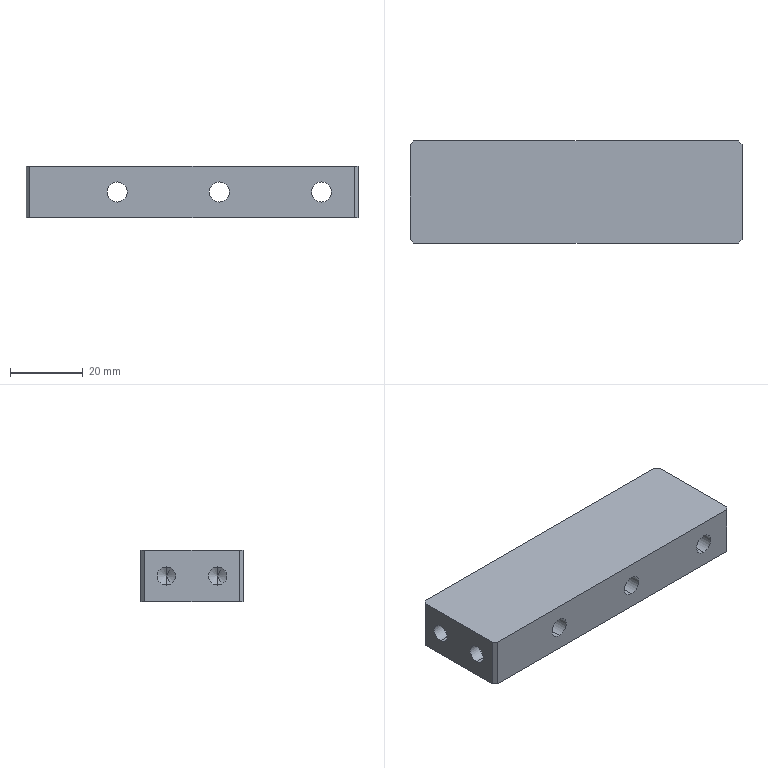Part | SolidWorks | features HoleWzd 2, Chamfer 1, Extrusion 1 | 1 solid | 33 faces | box 91 x 28 x 14 mm | volume 31396 mm3 | cylinder 16 | plane 13 | cone 4 | commonest cylinder face diameters 5.5 x6 10 x6 5 x4
STEP:
#1=CARTESIAN_POINT('',(-20.5,4.,-5.));
#2=VERTEX_POINT('',#1);
#3=CARTESIAN_POINT('',(-20.5,4.,5.));
#4=VERTEX_POINT('',#3);
#5=CARTESIAN_POINT('',(-20.5,4.,0.));
#6=DIRECTION('',(0.,1.,0.));
#7=DIRECTION('',(0.,0.,1.));
#8=AXIS2_PLACEMENT_3D('',#5,#6,#7);
#9=CIRCLE('',#8,5.);
#10=EDGE_CURVE('',#2,#4,#9,.T.);
#11=ORIENTED_EDGE('',*,*,#10,.F.);
#12=CARTESIAN_POINT('',(-20.5,14.,-5.));
#13=VERTEX_POINT('',#12);
#14=CARTESIAN_POINT('',(-20.5,14.,-5.));
#15=DIRECTION('',(0.,1.,0.));
#16=VECTOR('',#15,1000.);
#17=LINE('',#14,#16);
#18=EDGE_CURVE('',#2,#13,#17,.T.);
#19=ORIENTED_EDGE('',*,*,#18,.T.);
#20=CARTESIAN_POINT('',(-20.5,14.,5.));
#21=VERTEX_POINT('',#20);
#22=CARTESIAN_POINT('',(-20.5,14.,0.));
#23=DIRECTION('',(0.,1.,0.));
#24=DIRECTION('',(0.,0.,1.));
#25=AXIS2_PLACEMENT_3D('',#22,#23,#24);
#26=CIRCLE('',#25,5.);
#27=EDGE_CURVE('',#13,#21,#26,.T.);
#28=ORIENTED_EDGE('',*,*,#27,.T.);
#29=CARTESIAN_POINT('',(-20.5,14.,5.));
#30=DIRECTION('',(0.,1.,0.));
#31=VECTOR('',#30,1000.);
#32=LINE('',#29,#31);
#33=EDGE_CURVE('',#4,#21,#32,.T.);
#34=ORIENTED_EDGE('',*,*,#33,.F.);
#35=EDGE_LOOP('',(#11,#19,#28,#34));
#36=FACE_OUTER_BOUND('',#35,.T.);
#37=CARTESIAN_POINT('',(-20.5,14.,0.));
#38=DIRECTION('',(0.,1.,0.));
#39=DIRECTION('',(0.,0.,1.));
#40=AXIS2_PLACEMENT_3D('',#37,#38,#39);
#41=CYLINDRICAL_SURFACE('',#40,5.);
#42=ADVANCED_FACE('',(#36),#41,.F.);
#43=CARTESIAN_POINT('',(-20.5,-14.,-2.75));
#44=VERTEX_POINT('',#43);
#45=CARTESIAN_POINT('',(-20.5,-14.,2.75));
#46=VERTEX_POINT('',#45);
#47=CARTESIAN_POINT('',(-20.5,-14.,0.));
#48=DIRECTION('',(0.,1.,0.));
#49=DIRECTION('',(0.,0.,1.));
#50=AXIS2_PLACEMENT_3D('',#47,#48,#49);
#51=CIRCLE('',#50,2.75);
#52=EDGE_CURVE('',#44,#46,#51,.T.);
#53=ORIENTED_EDGE('',*,*,#52,.F.);
#54=CARTESIAN_POINT('',(-20.5,4.,-2.75));
#55=VERTEX_POINT('',#54);
#56=CARTESIAN_POINT('',(-20.5,14.,-2.75));
#57=DIRECTION('',(0.,1.,0.));
#58=VECTOR('',#57,1000.);
#59=LINE('',#56,#58);
#60=EDGE_CURVE('',#44,#55,#59,.T.);
#61=ORIENTED_EDGE('',*,*,#60,.T.);
#62=CARTESIAN_POINT('',(-20.5,4.,2.75));
#63=VERTEX_POINT('',#62);
#64=CARTESIAN_POINT('',(-20.5,4.,0.));
#65=DIRECTION('',(0.,1.,0.));
#66=DIRECTION('',(0.,0.,1.));
#67=AXIS2_PLACEMENT_3D('',#64,#65,#66);
#68=CIRCLE('',#67,2.75);
#69=EDGE_CURVE('',#55,#63,#68,.T.);
#70=ORIENTED_EDGE('',*,*,#69,.T.);
#71=CARTESIAN_POINT('',(-20.5,14.,2.75));
#72=DIRECTION('',(0.,1.,0.));
#73=VECTOR('',#72,1000.);
#74=LINE('',#71,#73);
#75=EDGE_CURVE('',#46,#63,#74,.T.);
#76=ORIENTED_EDGE('',*,*,#75,.F.);
#77=EDGE_LOOP('',(#53,#61,#70,#76));
#78=FACE_OUTER_BOUND('',#77,.T.);
#79=CARTESIAN_POINT('',(-20.5,14.,0.));
#80=DIRECTION('',(0.,1.,0.));
#81=DIRECTION('',(0.,0.,1.));
#82=AXIS2_PLACEMENT_3D('',#79,#80,#81);
#83=CYLINDRICAL_SURFACE('',#82,2.75);
#84=ADVANCED_FACE('',(#78),#83,.F.);
#85=CARTESIAN_POINT('',(35.5,4.,-5.));
#86=VERTEX_POINT('',#85);
#87=CARTESIAN_POINT('',(35.5,4.,5.));
#88=VERTEX_POINT('',#87);
#89=CARTESIAN_POINT('',(35.5,4.,0.));
#90=DIRECTION('',(0.,1.,0.));
#91=DIRECTION('',(0.,0.,1.));
#92=AXIS2_PLACEMENT_3D('',#89,#90,#91);
#93=CIRCLE('',#92,5.);
#94=EDGE_CURVE('',#86,#88,#93,.T.);
#95=ORIENTED_EDGE('',*,*,#94,.F.);
#96=CARTESIAN_POINT('',(35.5,14.,-5.));
#97=VERTEX_POINT('',#96);
#98=CARTESIAN_POINT('',(35.5,14.,-5.));
#99=DIRECTION('',(0.,1.,0.));
#100=VECTOR('',#99,1000.);
#101=LINE('',#98,#100);
#102=EDGE_CURVE('',#86,#97,#101,.T.);
#103=ORIENTED_EDGE('',*,*,#102,.T.);
#104=CARTESIAN_POINT('',(35.5,14.,5.));
#105=VERTEX_POINT('',#104);
#106=CARTESIAN_POINT('',(35.5,14.,0.));
#107=DIRECTION('',(0.,1.,0.));
#108=DIRECTION('',(0.,0.,1.));
#109=AXIS2_PLACEMENT_3D('',#106,#107,#108);
#110=CIRCLE('',#109,5.);
#111=EDGE_CURVE('',#97,#105,#110,.T.);
#112=ORIENTED_EDGE('',*,*,#111,.T.);
#113=CARTESIAN_POINT('',(35.5,14.,5.));
#114=DIRECTION('',(0.,1.,0.));
#115=VECTOR('',#114,1000.);
#116=LINE('',#113,#115);
#117=EDGE_CURVE('',#88,#105,#116,.T.);
#118=ORIENTED_EDGE('',*,*,#117,.F.);
#119=EDGE_LOOP('',(#95,#103,#112,#118));
#120=FACE_OUTER_BOUND('',#119,.T.);
#121=CARTESIAN_POINT('',(35.5,14.,0.));
#122=DIRECTION('',(0.,1.,0.));
#123=DIRECTION('',(0.,0.,1.));
#124=AXIS2_PLACEMENT_3D('',#121,#122,#123);
#125=CYLINDRICAL_SURFACE('',#124,5.);
#126=ADVANCED_FACE('',(#120),#125,.F.);
#127=CARTESIAN_POINT('',(35.5,-14.,-2.75));
#128=VERTEX_POINT('',#127);
#129=CARTESIAN_POINT('',(35.5,-14.,2.75));
#130=VERTEX_POINT('',#129);
#131=CARTESIAN_POINT('',(35.5,-14.,0.));
#132=DIRECTION('',(0.,1.,0.));
#133=DIRECTION('',(0.,0.,1.));
#134=AXIS2_PLACEMENT_3D('',#131,#132,#133);
#135=CIRCLE('',#134,2.75);
#136=EDGE_CURVE('',#128,#130,#135,.T.);
#137=ORIENTED_EDGE('',*,*,#136,.F.);
#138=CARTESIAN_POINT('',(35.5,4.,-2.75));
#139=VERTEX_POINT('',#138);
#140=CARTESIAN_POINT('',(35.5,14.,-2.75));
#141=DIRECTION('',(0.,1.,0.));
#142=VECTOR('',#141,1000.);
#143=LINE('',#140,#142);
#144=EDGE_CURVE('',#128,#139,#143,.T.);
#145=ORIENTED_EDGE('',*,*,#144,.T.);
#146=CARTESIAN_POINT('',(35.5,4.,2.75));
#147=VERTEX_POINT('',#146);
#148=CARTESIAN_POINT('',(35.5,4.,0.));
#149=DIRECTION('',(0.,1.,0.));
#150=DIRECTION('',(0.,0.,1.));
#151=AXIS2_PLACEMENT_3D('',#148,#149,#150);
#152=CIRCLE('',#151,2.75);
#153=EDGE_CURVE('',#139,#147,#152,.T.);
#154=ORIENTED_EDGE('',*,*,#153,.T.);
#155=CARTESIAN_POINT('',(35.5,14.,2.75));
#156=DIRECTION('',(0.,1.,0.));
#157=VECTOR('',#156,1000.);
#158=LINE('',#155,#157);
#159=EDGE_CURVE('',#130,#147,#158,.T.);
#160=ORIENTED_EDGE('',*,*,#159,.F.);
#161=EDGE_LOOP('',(#137,#145,#154,#160));
#162=FACE_OUTER_BOUND('',#161,.T.);
#163=CARTESIAN_POINT('',(35.5,14.,0.));
#164=DIRECTION('',(0.,1.,0.));
#165=DIRECTION('',(0.,0.,1.));
#166=AXIS2_PLACEMENT_3D('',#163,#164,#165);
#167=CYLINDRICAL_SURFACE('',#166,2.75);
#168=ADVANCED_FACE('',(#162),#167,.F.);
#169=CARTESIAN_POINT('',(7.5,4.,-5.));
#170=VERTEX_POINT('',#169);
#171=CARTESIAN_POINT('',(7.5,4.,5.));
#172=VERTEX_POINT('',#171);
#173=CARTESIAN_POINT('',(7.5,4.,0.));
#174=DIRECTION('',(0.,1.,0.));
#175=DIRECTION('',(0.,0.,1.));
#176=AXIS2_PLACEMENT_3D('',#173,#174,#175);
#177=CIRCLE('',#176,5.);
#178=EDGE_CURVE('',#170,#172,#177,.T.);
#179=ORIENTED_EDGE('',*,*,#178,.F.);
#180=CARTESIAN_POINT('',(7.5,14.,-5.));
#181=VERTEX_POINT('',#180);
#182=CARTESIAN_POINT('',(7.5,14.,-5.));
#183=DIRECTION('',(0.,1.,0.));
#184=VECTOR('',#183,1000.);
#185=LINE('',#182,#184);
#186=EDGE_CURVE('',#170,#181,#185,.T.);
#187=ORIENTED_EDGE('',*,*,#186,.T.);
#188=CARTESIAN_POINT('',(7.5,14.,5.));
#189=VERTEX_POINT('',#188);
#190=CARTESIAN_POINT('',(7.5,14.,0.));
#191=DIRECTION('',(0.,1.,0.));
#192=DIRECTION('',(0.,0.,1.));
#193=AXIS2_PLACEMENT_3D('',#190,#191,#192);
#194=CIRCLE('',#193,5.);
#195=EDGE_CURVE('',#181,#189,#194,.T.);
#196=ORIENTED_EDGE('',*,*,#195,.T.);
#197=CARTESIAN_POINT('',(7.5,14.,5.));
#198=DIRECTION('',(0.,1.,0.));
#199=VECTOR('',#198,1000.);
#200=LINE('',#197,#199);
#201=EDGE_CURVE('',#172,#189,#200,.T.);
#202=ORIENTED_EDGE('',*,*,#201,.F.);
#203=EDGE_LOOP('',(#179,#187,#196,#202));
#204=FACE_OUTER_BOUND('',#203,.T.);
#205=CARTESIAN_POINT('',(7.5,14.,0.));
#206=DIRECTION('',(0.,1.,0.));
#207=DIRECTION('',(0.,0.,1.));
#208=AXIS2_PLACEMENT_3D('',#205,#206,#207);
#209=CYLINDRICAL_SURFACE('',#208,5.);
#210=ADVANCED_FACE('',(#204),#209,.F.);
#211=CARTESIAN_POINT('',(7.5,-14.,-2.75));
#212=VERTEX_POINT('',#211);
#213=CARTESIAN_POINT('',(7.5,-14.,2.75));
#214=VERTEX_POINT('',#213);
#215=CARTESIAN_POINT('',(7.5,-14.,0.));
#216=DIRECTION('',(0.,1.,0.));
#217=DIRECTION('',(0.,0.,1.));
#218=AXIS2_PLACEMENT_3D('',#215,#216,#217);
#219=CIRCLE('',#218,2.75);
#220=EDGE_CURVE('',#212,#214,#219,.T.);
#221=ORIENTED_EDGE('',*,*,#220,.F.);
#222=CARTESIAN_POINT('',(7.5,4.,-2.75));
#223=VERTEX_POINT('',#222);
#224=CARTESIAN_POINT('',(7.5,14.,-2.75));
#225=DIRECTION('',(0.,1.,0.));
#226=VECTOR('',#225,1000.);
#227=LINE('',#224,#226);
#228=EDGE_CURVE('',#212,#223,#227,.T.);
#229=ORIENTED_EDGE('',*,*,#228,.T.);
#230=CARTESIAN_POINT('',(7.5,4.,2.75));
#231=VERTEX_POINT('',#230);
#232=CARTESIAN_POINT('',(7.5,4.,0.));
#233=DIRECTION('',(0.,1.,0.));
#234=DIRECTION('',(0.,0.,1.));
#235=AXIS2_PLACEMENT_3D('',#232,#233,#234);
#236=CIRCLE('',#235,2.75);
#237=EDGE_CURVE('',#223,#231,#236,.T.);
#238=ORIENTED_EDGE('',*,*,#237,.T.);
#239=CARTESIAN_POINT('',(7.5,14.,2.75));
#240=DIRECTION('',(0.,1.,0.));
#241=VECTOR('',#240,1000.);
#242=LINE('',#239,#241);
#243=EDGE_CURVE('',#214,#231,#242,.T.);
#244=ORIENTED_EDGE('',*,*,#243,.F.);
#245=EDGE_LOOP('',(#221,#229,#238,#244));
#246=FACE_OUTER_BOUND('',#245,.T.);
#247=CARTESIAN_POINT('',(7.5,14.,0.));
#248=DIRECTION('',(0.,1.,0.));
#249=DIRECTION('',(0.,0.,1.));
#250=AXIS2_PLACEMENT_3D('',#247,#248,#249);
#251=CYLINDRICAL_SURFACE('',#250,2.75);
#252=ADVANCED_FACE('',(#246),#251,.F.);
#253=CARTESIAN_POINT('',(-30.5,7.,-2.5));
#254=VERTEX_POINT('',#253);
#255=CARTESIAN_POINT('',(-30.5,7.,2.5));
#256=VERTEX_POINT('',#255);
#257=CARTESIAN_POINT('',(-30.5,7.,0.));
#258=DIRECTION('',(-1.,0.,0.));
#259=DIRECTION('',(0.,0.,1.));
#260=AXIS2_PLACEMENT_3D('',#257,#258,#259);
#261=CIRCLE('',#260,2.5);
#262=EDGE_CURVE('',#254,#256,#261,.T.);
#263=ORIENTED_EDGE('',*,*,#262,.F.);
#264=CARTESIAN_POINT('',(-45.5,7.,-2.5));
#265=VERTEX_POINT('',#264);
#266=CARTESIAN_POINT('',(-45.5,7.,-2.5));
#267=DIRECTION('',(-1.,0.,0.));
#268=VECTOR('',#267,1000.);
#269=LINE('',#266,#268);
#270=EDGE_CURVE('',#254,#265,#269,.T.);
#271=ORIENTED_EDGE('',*,*,#270,.T.);
#272=CARTESIAN_POINT('',(-45.5,7.,2.5));
#273=VERTEX_POINT('',#272);
#274=CARTESIAN_POINT('',(-45.5,7.,0.));
#275=DIRECTION('',(-1.,0.,0.));
#276=DIRECTION('',(0.,0.,1.));
#277=AXIS2_PLACEMENT_3D('',#274,#275,#276);
#278=CIRCLE('',#277,2.5);
#279=EDGE_CURVE('',#265,#273,#278,.T.);
#280=ORIENTED_EDGE('',*,*,#279,.T.);
#281=CARTESIAN_POINT('',(-45.5,7.,2.5));
#282=DIRECTION('',(-1.,0.,0.));
#283=VECTOR('',#282,1000.);
#284=LINE('',#281,#283);
#285=EDGE_CURVE('',#256,#273,#284,.T.);
#286=ORIENTED_EDGE('',*,*,#285,.F.);
#287=EDGE_LOOP('',(#263,#271,#280,#286));
#288=FACE_OUTER_BOUND('',#287,.T.);
#289=CARTESIAN_POINT('',(-45.5,7.,0.));
#290=DIRECTION('',(-1.,0.,0.));
#291=DIRECTION('',(0.,0.,1.));
#292=AXIS2_PLACEMENT_3D('',#289,#290,#291);
#293=CYLINDRICAL_SURFACE('',#292,2.5);
#294=ADVANCED_FACE('',(#288),#293,.F.);
#295=CARTESIAN_POINT('',(-28.998,7.,0.));
#296=VERTEX_POINT('',#295);
#297=CARTESIAN_POINT('',(-30.5,7.,2.5));
#298=DIRECTION('',(-0.515,0.,0.8572));
#299=VECTOR('',#298,1000.);
#300=LINE('',#297,#299);
#301=EDGE_CURVE('',#296,#256,#300,.T.);
#302=ORIENTED_EDGE('',*,*,#301,.F.);
#303=CARTESIAN_POINT('',(-30.5,7.,-2.5));
#304=DIRECTION('',(-0.515,0.,-0.8572));
#305=VECTOR('',#304,1000.);
#306=LINE('',#303,#305);
#307=EDGE_CURVE('',#296,#254,#306,.T.);
#308=ORIENTED_EDGE('',*,*,#307,.T.);
#309=ORIENTED_EDGE('',*,*,#262,.T.);
#310=EDGE_LOOP('',(#302,#308,#309));
#311=FACE_OUTER_BOUND('',#310,.T.);
#312=CARTESIAN_POINT('',(-30.5,7.,0.));
#313=DIRECTION('',(-1.,0.,0.));
#314=DIRECTION('',(0.,0.,1.));
#315=AXIS2_PLACEMENT_3D('',#312,#313,#314);
#316=CONICAL_SURFACE('',#315,2.5,1.03);
#317=ADVANCED_FACE('',(#311),#316,.F.);
#318=CARTESIAN_POINT('',(-30.5,-7.,-2.5));
#319=VERTEX_POINT('',#318);
#320=CARTESIAN_POINT('',(-30.5,-7.,2.5));
#321=VERTEX_POINT('',#320);
#322=CARTESIAN_POINT('',(-30.5,-7.,0.));
#323=DIRECTION('',(-1.,0.,0.));
#324=DIRECTION('',(0.,0.,1.));
#325=AXIS2_PLACEMENT_3D('',#322,#323,#324);
#326=CIRCLE('',#325,2.5);
#327=EDGE_CURVE('',#319,#321,#326,.T.);
#328=ORIENTED_EDGE('',*,*,#327,.F.);
#329=CARTESIAN_POINT('',(-45.5,-7.,-2.5));
#330=VERTEX_POINT('',#329);
#331=CARTESIAN_POINT('',(-45.5,-7.,-2.5));
#332=DIRECTION('',(-1.,0.,0.));
#333=VECTOR('',#332,1000.);
#334=LINE('',#331,#333);
#335=EDGE_CURVE('',#319,#330,#334,.T.);
#336=ORIENTED_EDGE('',*,*,#335,.T.);
#337=CARTESIAN_POINT('',(-45.5,-7.,2.5));
#338=VERTEX_POINT('',#337);
#339=CARTESIAN_POINT('',(-45.5,-7.,0.));
#340=DIRECTION('',(-1.,0.,0.));
#341=DIRECTION('',(0.,0.,1.));
#342=AXIS2_PLACEMENT_3D('',#339,#340,#341);
#343=CIRCLE('',#342,2.5);
#344=EDGE_CURVE('',#330,#338,#343,.T.);
#345=ORIENTED_EDGE('',*,*,#344,.T.);
#346=CARTESIAN_POINT('',(-45.5,-7.,2.5));
#347=DIRECTION('',(-1.,0.,0.));
#348=VECTOR('',#347,1000.);
#349=LINE('',#346,#348);
#350=EDGE_CURVE('',#321,#338,#349,.T.);
#351=ORIENTED_EDGE('',*,*,#350,.F.);
#352=EDGE_LOOP('',(#328,#336,#345,#351));
#353=FACE_OUTER_BOUND('',#352,.T.);
#354=CARTESIAN_POINT('',(-45.5,-7.,0.));
#355=DIRECTION('',(-1.,0.,0.));
#356=DIRECTION('',(0.,0.,1.));
#357=AXIS2_PLACEMENT_3D('',#354,#355,#356);
#358=CYLINDRICAL_SURFACE('',#357,2.5);
#359=ADVANCED_FACE('',(#353),#358,.F.);
#360=CARTESIAN_POINT('',(-28.998,-7.,0.));
#361=VERTEX_POINT('',#360);
#362=CARTESIAN_POINT('',(-30.5,-7.,2.5));
#363=DIRECTION('',(-0.515,0.,0.8572));
#364=VECTOR('',#363,1000.);
#365=LINE('',#362,#364);
#366=EDGE_CURVE('',#361,#321,#365,.T.);
#367=ORIENTED_EDGE('',*,*,#366,.F.);
#368=CARTESIAN_POINT('',(-30.5,-7.,-2.5));
#369=DIRECTION('',(-0.515,0.,-0.8572));
#370=VECTOR('',#369,1000.);
#371=LINE('',#368,#370);
#372=EDGE_CURVE('',#361,#319,#371,.T.);
#373=ORIENTED_EDGE('',*,*,#372,.T.);
#374=ORIENTED_EDGE('',*,*,#327,.T.);
#375=EDGE_LOOP('',(#367,#373,#374));
#376=FACE_OUTER_BOUND('',#375,.T.);
#377=CARTESIAN_POINT('',(-30.5,-7.,0.));
#378=DIRECTION('',(-1.,0.,0.));
#379=DIRECTION('',(0.,0.,1.));
#380=AXIS2_PLACEMENT_3D('',#377,#378,#379);
#381=CONICAL_SURFACE('',#380,2.5,1.03);
#382=ADVANCED_FACE('',(#376),#381,.F.);
#383=CARTESIAN_POINT('',(45.5,-13.,-7.));
#384=VERTEX_POINT('',#383);
#385=CARTESIAN_POINT('',(45.5,13.,-7.));
#386=VERTEX_POINT('',#385);
#387=CARTESIAN_POINT('',(45.5,-14.,-7.));
#388=DIRECTION('',(0.,1.,0.));
#389=VECTOR('',#388,1000.);
#390=LINE('',#387,#389);
#391=EDGE_CURVE('',#384,#386,#390,.T.);
#392=ORIENTED_EDGE('',*,*,#391,.T.);
#393=CARTESIAN_POINT('',(45.5,13.,7.));
#394=VERTEX_POINT('',#393);
#395=CARTESIAN_POINT('',(45.5,13.,7.));
#396=DIRECTION('',(0.,0.,1.));
#397=VECTOR('',#396,1000.);
#398=LINE('',#395,#397);
#399=EDGE_CURVE('',#386,#394,#398,.T.);
#400=ORIENTED_EDGE('',*,*,#399,.T.);
#401=CARTESIAN_POINT('',(45.5,-13.,7.));
#402=VERTEX_POINT('',#401);
#403=CARTESIAN_POINT('',(45.5,-14.,7.));
#404=DIRECTION('',(0.,1.,0.));
#405=VECTOR('',#404,1000.);
#406=LINE('',#403,#405);
#407=EDGE_CURVE('',#402,#394,#406,.T.);
#408=ORIENTED_EDGE('',*,*,#407,.F.);
#409=CARTESIAN_POINT('',(45.5,-13.,7.));
#410=DIRECTION('',(0.,0.,-1.));
#411=VECTOR('',#410,1000.);
#412=LINE('',#409,#411);
#413=EDGE_CURVE('',#402,#384,#412,.T.);
#414=ORIENTED_EDGE('',*,*,#413,.T.);
#415=EDGE_LOOP('',(#392,#400,#408,#414));
#416=FACE_OUTER_BOUND('',#415,.T.);
#417=CARTESIAN_POINT('',(45.5,-14.,7.));
#418=DIRECTION('',(-1.,0.,0.));
#419=DIRECTION('',(0.,0.,1.));
#420=AXIS2_PLACEMENT_3D('',#417,#418,#419);
#421=PLANE('',#420);
#422=ADVANCED_FACE('',(#416),#421,.F.);
#423=CARTESIAN_POINT('',(-20.5,14.,0.));
#424=DIRECTION('',(0.,1.,0.));
#425=DIRECTION('',(0.,0.,1.));
#426=AXIS2_PLACEMENT_3D('',#423,#424,#425);
#427=CIRCLE('',#426,5.);
#428=EDGE_CURVE('',#21,#13,#427,.T.);
#429=ORIENTED_EDGE('',*,*,#428,.F.);
#430=ORIENTED_EDGE('',*,*,#27,.F.);
#431=EDGE_LOOP('',(#429,#430));
#432=FACE_BOUND('',#431,.T.);
#433=CARTESIAN_POINT('',(35.5,14.,0.));
#434=DIRECTION('',(0.,1.,0.));
#435=DIRECTION('',(0.,0.,1.));
#436=AXIS2_PLACEMENT_3D('',#433,#434,#435);
#437=CIRCLE('',#436,5.);
#438=EDGE_CURVE('',#105,#97,#437,.T.);
#439=ORIENTED_EDGE('',*,*,#438,.F.);
#440=ORIENTED_EDGE('',*,*,#111,.F.);
#441=EDGE_LOOP('',(#439,#440));
#442=FACE_BOUND('',#441,.T.);
#443=CARTESIAN_POINT('',(7.5,14.,0.));
#444=DIRECTION('',(0.,1.,0.));
#445=DIRECTION('',(0.,0.,1.));
#446=AXIS2_PLACEMENT_3D('',#443,#444,#445);
#447=CIRCLE('',#446,5.);
#448=EDGE_CURVE('',#189,#181,#447,.T.);
#449=ORIENTED_EDGE('',*,*,#448,.F.);
#450=ORIENTED_EDGE('',*,*,#195,.F.);
#451=EDGE_LOOP('',(#449,#450));
#452=FACE_BOUND('',#451,.T.);
#453=CARTESIAN_POINT('',(44.5,14.,7.));
#454=VERTEX_POINT('',#453);
#455=CARTESIAN_POINT('',(-44.5,14.,7.));
#456=VERTEX_POINT('',#455);
#457=CARTESIAN_POINT('',(-45.5,14.,7.));
#458=DIRECTION('',(-1.,0.,0.));
#459=VECTOR('',#458,1000.);
#460=LINE('',#457,#459);
#461=EDGE_CURVE('',#454,#456,#460,.T.);
#462=ORIENTED_EDGE('',*,*,#461,.F.);
#463=CARTESIAN_POINT('',(44.5,14.,-7.));
#464=VERTEX_POINT('',#463);
#465=CARTESIAN_POINT('',(44.5,14.,7.));
#466=DIRECTION('',(0.,0.,-1.));
#467=VECTOR('',#466,1000.);
#468=LINE('',#465,#467);
#469=EDGE_CURVE('',#454,#464,#468,.T.);
#470=ORIENTED_EDGE('',*,*,#469,.T.);
#471=CARTESIAN_POINT('',(-44.5,14.,-7.));
#472=VERTEX_POINT('',#471);
#473=CARTESIAN_POINT('',(-45.5,14.,-7.));
#474=DIRECTION('',(-1.,0.,0.));
#475=VECTOR('',#474,1000.);
#476=LINE('',#473,#475);
#477=EDGE_CURVE('',#464,#472,#476,.T.);
#478=ORIENTED_EDGE('',*,*,#477,.T.);
#479=CARTESIAN_POINT('',(-44.5,14.,7.));
#480=DIRECTION('',(0.,0.,1.));
#481=VECTOR('',#480,1000.);
#482=LINE('',#479,#481);
#483=EDGE_CURVE('',#472,#456,#482,.T.);
#484=ORIENTED_EDGE('',*,*,#483,.T.);
#485=EDGE_LOOP('',(#462,#470,#478,#484));
#486=FACE_OUTER_BOUND('',#485,.T.);
#487=CARTESIAN_POINT('',(-45.5,14.,7.));
#488=DIRECTION('',(0.,-1.,0.));
#489=DIRECTION('',(0.,0.,-1.));
#490=AXIS2_PLACEMENT_3D('',#487,#488,#489);
#491=PLANE('',#490);
#492=ADVANCED_FACE('',(#432,#442,#452,#486),#491,.F.);
#493=CARTESIAN_POINT('',(-45.5,7.,0.));
#494=DIRECTION('',(-1.,0.,0.));
#495=DIRECTION('',(0.,0.,1.));
#496=AXIS2_PLACEMENT_3D('',#493,#494,#495);
#497=CIRCLE('',#496,2.5);
#498=EDGE_CURVE('',#273,#265,#497,.T.);
#499=ORIENTED_EDGE('',*,*,#498,.F.);
#500=ORIENTED_EDGE('',*,*,#279,.F.);
#501=EDGE_LOOP('',(#499,#500));
#502=FACE_BOUND('',#501,.T.);
#503=CARTESIAN_POINT('',(-45.5,-7.,0.));
#504=DIRECTION('',(-1.,0.,0.));
#505=DIRECTION('',(0.,0.,1.));
#506=AXIS2_PLACEMENT_3D('',#503,#504,#505);
#507=CIRCLE('',#506,2.5);
#508=EDGE_CURVE('',#338,#330,#507,.T.);
#509=ORIENTED_EDGE('',*,*,#508,.F.);
#510=ORIENTED_EDGE('',*,*,#344,.F.);
#511=EDGE_LOOP('',(#509,#510));
#512=FACE_BOUND('',#511,.T.);
#513=CARTESIAN_POINT('',(-45.5,13.,-7.));
#514=VERTEX_POINT('',#513);
#515=CARTESIAN_POINT('',(-45.5,-13.,-7.));
#516=VERTEX_POINT('',#515);
#517=CARTESIAN_POINT('',(-45.5,-14.,-7.));
#518=DIRECTION('',(0.,-1.,0.));
#519=VECTOR('',#518,1000.);
#520=LINE('',#517,#519);
#521=EDGE_CURVE('',#514,#516,#520,.T.);
#522=ORIENTED_EDGE('',*,*,#521,.T.);
#523=CARTESIAN_POINT('',(-45.5,-13.,7.));
#524=VERTEX_POINT('',#523);
#525=CARTESIAN_POINT('',(-45.5,-13.,7.));
#526=DIRECTION('',(0.,0.,1.));
#527=VECTOR('',#526,1000.);
#528=LINE('',#525,#527);
#529=EDGE_CURVE('',#516,#524,#528,.T.);
#530=ORIENTED_EDGE('',*,*,#529,.T.);
#531=CARTESIAN_POINT('',(-45.5,13.,7.));
#532=VERTEX_POINT('',#531);
#533=CARTESIAN_POINT('',(-45.5,-14.,7.));
#534=DIRECTION('',(0.,-1.,0.));
#535=VECTOR('',#534,1000.);
#536=LINE('',#533,#535);
#537=EDGE_CURVE('',#532,#524,#536,.T.);
#538=ORIENTED_EDGE('',*,*,#537,.F.);
#539=CARTESIAN_POINT('',(-45.5,13.,7.));
#540=DIRECTION('',(0.,0.,-1.));
#541=VECTOR('',#540,1000.);
#542=LINE('',#539,#541);
#543=EDGE_CURVE('',#532,#514,#542,.T.);
#544=ORIENTED_EDGE('',*,*,#543,.T.);
#545=EDGE_LOOP('',(#522,#530,#538,#544));
#546=FACE_OUTER_BOUND('',#545,.T.);
#547=CARTESIAN_POINT('',(-45.5,-14.,7.));
#548=DIRECTION('',(1.,0.,0.));
#549=DIRECTION('',(0.,0.,-1.));
#550=AXIS2_PLACEMENT_3D('',#547,#548,#549);
#551=PLANE('',#550);
#552=ADVANCED_FACE('',(#502,#512,#546),#551,.F.);
#553=CARTESIAN_POINT('',(-20.5,-14.,0.));
#554=DIRECTION('',(0.,1.,0.));
#555=DIRECTION('',(0.,0.,1.));
#556=AXIS2_PLACEMENT_3D('',#553,#554,#555);
#557=CIRCLE('',#556,2.75);
#558=EDGE_CURVE('',#46,#44,#557,.T.);
#559=ORIENTED_EDGE('',*,*,#558,.T.);
#560=ORIENTED_EDGE('',*,*,#52,.T.);
#561=EDGE_LOOP('',(#559,#560));
#562=FACE_BOUND('',#561,.T.);
#563=CARTESIAN_POINT('',(35.5,-14.,0.));
#564=DIRECTION('',(0.,1.,0.));
#565=DIRECTION('',(0.,0.,1.));
#566=AXIS2_PLACEMENT_3D('',#563,#564,#565);
#567=CIRCLE('',#566,2.75);
#568=EDGE_CURVE('',#130,#128,#567,.T.);
#569=ORIENTED_EDGE('',*,*,#568,.T.);
#570=ORIENTED_EDGE('',*,*,#136,.T.);
#571=EDGE_LOOP('',(#569,#570));
#572=FACE_BOUND('',#571,.T.);
#573=CARTESIAN_POINT('',(7.5,-14.,0.));
#574=DIRECTION('',(0.,1.,0.));
#575=DIRECTION('',(0.,0.,1.));
#576=AXIS2_PLACEMENT_3D('',#573,#574,#575);
#577=CIRCLE('',#576,2.75);
#578=EDGE_CURVE('',#214,#212,#577,.T.);
#579=ORIENTED_EDGE('',*,*,#578,.T.);
#580=ORIENTED_EDGE('',*,*,#220,.T.);
#581=EDGE_LOOP('',(#579,#580));
#582=FACE_BOUND('',#581,.T.);
#583=CARTESIAN_POINT('',(-44.5,-14.,-7.));
#584=VERTEX_POINT('',#583);
#585=CARTESIAN_POINT('',(44.5,-14.,-7.));
#586=VERTEX_POINT('',#585);
#587=CARTESIAN_POINT('',(-45.5,-14.,-7.));
#588=DIRECTION('',(1.,0.,0.));
#589=VECTOR('',#588,1000.);
#590=LINE('',#587,#589);
#591=EDGE_CURVE('',#584,#586,#590,.T.);
#592=ORIENTED_EDGE('',*,*,#591,.T.);
#593=CARTESIAN_POINT('',(44.5,-14.,7.));
#594=VERTEX_POINT('',#593);
#595=CARTESIAN_POINT('',(44.5,-14.,7.));
#596=DIRECTION('',(0.,0.,1.));
#597=VECTOR('',#596,1000.);
#598=LINE('',#595,#597);
#599=EDGE_CURVE('',#586,#594,#598,.T.);
#600=ORIENTED_EDGE('',*,*,#599,.T.);
#601=CARTESIAN_POINT('',(-44.5,-14.,7.));
#602=VERTEX_POINT('',#601);
#603=CARTESIAN_POINT('',(-45.5,-14.,7.));
#604=DIRECTION('',(1.,0.,0.));
#605=VECTOR('',#604,1000.);
#606=LINE('',#603,#605);
#607=EDGE_CURVE('',#602,#594,#606,.T.);
#608=ORIENTED_EDGE('',*,*,#607,.F.);
#609=CARTESIAN_POINT('',(-44.5,-14.,7.));
#610=DIRECTION('',(0.,0.,-1.));
#611=VECTOR('',#610,1000.);
#612=LINE('',#609,#611);
#613=EDGE_CURVE('',#602,#584,#612,.T.);
#614=ORIENTED_EDGE('',*,*,#613,.T.);
#615=EDGE_LOOP('',(#592,#600,#608,#614));
#616=FACE_OUTER_BOUND('',#615,.T.);
#617=CARTESIAN_POINT('',(-45.5,-14.,7.));
#618=DIRECTION('',(0.,1.,0.));
#619=DIRECTION('',(0.,0.,1.));
#620=AXIS2_PLACEMENT_3D('',#617,#618,#619);
#621=PLANE('',#620);
#622=ADVANCED_FACE('',(#562,#572,#582,#616),#621,.F.);
#623=ORIENTED_EDGE('',*,*,#407,.T.);
#624=CARTESIAN_POINT('',(44.5,14.,7.));
#625=DIRECTION('',(-0.7071,0.7071,0.));
#626=VECTOR('',#625,1000.);
#627=LINE('',#624,#626);
#628=EDGE_CURVE('',#394,#454,#627,.T.);
#629=ORIENTED_EDGE('',*,*,#628,.T.);
#630=ORIENTED_EDGE('',*,*,#461,.T.);
#631=CARTESIAN_POINT('',(-45.5,13.,7.));
#632=DIRECTION('',(-0.7071,-0.7071,0.));
#633=VECTOR('',#632,1000.);
#634=LINE('',#631,#633);
#635=EDGE_CURVE('',#456,#532,#634,.T.);
#636=ORIENTED_EDGE('',*,*,#635,.T.);
#637=ORIENTED_EDGE('',*,*,#537,.T.);
#638=CARTESIAN_POINT('',(-44.5,-14.,7.));
#639=DIRECTION('',(0.7071,-0.7071,0.));
#640=VECTOR('',#639,1000.);
#641=LINE('',#638,#640);
#642=EDGE_CURVE('',#524,#602,#641,.T.);
#643=ORIENTED_EDGE('',*,*,#642,.T.);
#644=ORIENTED_EDGE('',*,*,#607,.T.);
#645=CARTESIAN_POINT('',(45.5,-13.,7.));
#646=DIRECTION('',(0.7071,0.7071,0.));
#647=VECTOR('',#646,1000.);
#648=LINE('',#645,#647);
#649=EDGE_CURVE('',#594,#402,#648,.T.);
#650=ORIENTED_EDGE('',*,*,#649,.T.);
#651=EDGE_LOOP('',(#623,#629,#630,#636,#637,#643,#644,#650));
#652=FACE_OUTER_BOUND('',#651,.T.);
#653=CARTESIAN_POINT('',(0.,0.,7.));
#654=DIRECTION('',(0.,0.,-1.));
#655=DIRECTION('',(-1.,0.,0.));
#656=AXIS2_PLACEMENT_3D('',#653,#654,#655);
#657=PLANE('',#656);
#658=ADVANCED_FACE('',(#652),#657,.F.);
#659=ORIENTED_EDGE('',*,*,#477,.F.);
#660=CARTESIAN_POINT('',(29.25,29.25,-7.));
#661=DIRECTION('',(0.7071,-0.7071,0.));
#662=VECTOR('',#661,1000.);
#663=LINE('',#660,#662);
#664=EDGE_CURVE('',#464,#386,#663,.T.);
#665=ORIENTED_EDGE('',*,*,#664,.T.);
#666=ORIENTED_EDGE('',*,*,#391,.F.);
#667=CARTESIAN_POINT('',(29.25,-29.25,-7.));
#668=DIRECTION('',(-0.7071,-0.7071,0.));
#669=VECTOR('',#668,1000.);
#670=LINE('',#667,#669);
#671=EDGE_CURVE('',#384,#586,#670,.T.);
#672=ORIENTED_EDGE('',*,*,#671,.T.);
#673=ORIENTED_EDGE('',*,*,#591,.F.);
#674=CARTESIAN_POINT('',(-29.25,-29.25,-7.));
#675=DIRECTION('',(-0.7071,0.7071,0.));
#676=VECTOR('',#675,1000.);
#677=LINE('',#674,#676);
#678=EDGE_CURVE('',#584,#516,#677,.T.);
#679=ORIENTED_EDGE('',*,*,#678,.T.);
#680=ORIENTED_EDGE('',*,*,#521,.F.);
#681=CARTESIAN_POINT('',(-29.25,29.25,-7.));
#682=DIRECTION('',(0.7071,0.7071,0.));
#683=VECTOR('',#682,1000.);
#684=LINE('',#681,#683);
#685=EDGE_CURVE('',#514,#472,#684,.T.);
#686=ORIENTED_EDGE('',*,*,#685,.T.);
#687=EDGE_LOOP('',(#659,#665,#666,#672,#673,#679,#680,#686));
#688=FACE_OUTER_BOUND('',#687,.T.);
#689=CARTESIAN_POINT('',(0.,0.,-7.));
#690=DIRECTION('',(0.,0.,-1.));
#691=DIRECTION('',(-1.,0.,0.));
#692=AXIS2_PLACEMENT_3D('',#689,#690,#691);
#693=PLANE('',#692);
#694=ADVANCED_FACE('',(#688),#693,.T.);
#695=ORIENTED_EDGE('',*,*,#372,.F.);
#696=ORIENTED_EDGE('',*,*,#366,.T.);
#697=CARTESIAN_POINT('',(-30.5,-7.,0.));
#698=DIRECTION('',(-1.,0.,0.));
#699=DIRECTION('',(0.,0.,1.));
#700=AXIS2_PLACEMENT_3D('',#697,#698,#699);
#701=CIRCLE('',#700,2.5);
#702=EDGE_CURVE('',#321,#319,#701,.T.);
#703=ORIENTED_EDGE('',*,*,#702,.T.);
#704=EDGE_LOOP('',(#695,#696,#703));
#705=FACE_OUTER_BOUND('',#704,.T.);
#706=CARTESIAN_POINT('',(-30.5,-7.,0.));
#707=DIRECTION('',(-1.,0.,0.));
#708=DIRECTION('',(0.,0.,1.));
#709=AXIS2_PLACEMENT_3D('',#706,#707,#708);
#710=CONICAL_SURFACE('',#709,2.5,1.03);
#711=ADVANCED_FACE('',(#705),#710,.F.);
#712=ORIENTED_EDGE('',*,*,#335,.F.);
#713=ORIENTED_EDGE('',*,*,#702,.F.);
#714=ORIENTED_EDGE('',*,*,#350,.T.);
#715=ORIENTED_EDGE('',*,*,#508,.T.);
#716=EDGE_LOOP('',(#712,#713,#714,#715));
#717=FACE_OUTER_BOUND('',#716,.T.);
#718=CARTESIAN_POINT('',(-45.5,-7.,0.));
#719=DIRECTION('',(-1.,0.,0.));
#720=DIRECTION('',(0.,0.,1.));
#721=AXIS2_PLACEMENT_3D('',#718,#719,#720);
#722=CYLINDRICAL_SURFACE('',#721,2.5);
#723=ADVANCED_FACE('',(#717),#722,.F.);
#724=ORIENTED_EDGE('',*,*,#307,.F.);
#725=ORIENTED_EDGE('',*,*,#301,.T.);
#726=CARTESIAN_POINT('',(-30.5,7.,0.));
#727=DIRECTION('',(-1.,0.,0.));
#728=DIRECTION('',(0.,0.,1.));
#729=AXIS2_PLACEMENT_3D('',#726,#727,#728);
#730=CIRCLE('',#729,2.5);
#731=EDGE_CURVE('',#256,#254,#730,.T.);
#732=ORIENTED_EDGE('',*,*,#731,.T.);
#733=EDGE_LOOP('',(#724,#725,#732));
#734=FACE_OUTER_BOUND('',#733,.T.);
#735=CARTESIAN_POINT('',(-30.5,7.,0.));
#736=DIRECTION('',(-1.,0.,0.));
#737=DIRECTION('',(0.,0.,1.));
#738=AXIS2_PLACEMENT_3D('',#735,#736,#737);
#739=CONICAL_SURFACE('',#738,2.5,1.03);
#740=ADVANCED_FACE('',(#734),#739,.F.);
#741=ORIENTED_EDGE('',*,*,#270,.F.);
#742=ORIENTED_EDGE('',*,*,#731,.F.);
#743=ORIENTED_EDGE('',*,*,#285,.T.);
#744=ORIENTED_EDGE('',*,*,#498,.T.);
#745=EDGE_LOOP('',(#741,#742,#743,#744));
#746=FACE_OUTER_BOUND('',#745,.T.);
#747=CARTESIAN_POINT('',(-45.5,7.,0.));
#748=DIRECTION('',(-1.,0.,0.));
#749=DIRECTION('',(0.,0.,1.));
#750=AXIS2_PLACEMENT_3D('',#747,#748,#749);
#751=CYLINDRICAL_SURFACE('',#750,2.5);
#752=ADVANCED_FACE('',(#746),#751,.F.);
#753=ORIENTED_EDGE('',*,*,#228,.F.);
#754=ORIENTED_EDGE('',*,*,#578,.F.);
#755=ORIENTED_EDGE('',*,*,#243,.T.);
#756=CARTESIAN_POINT('',(7.5,4.,0.));
#757=DIRECTION('',(0.,1.,0.));
#758=DIRECTION('',(0.,0.,1.));
#759=AXIS2_PLACEMENT_3D('',#756,#757,#758);
#760=CIRCLE('',#759,2.75);
#761=EDGE_CURVE('',#231,#223,#760,.T.);
#762=ORIENTED_EDGE('',*,*,#761,.T.);
#763=EDGE_LOOP('',(#753,#754,#755,#762));
#764=FACE_OUTER_BOUND('',#763,.T.);
#765=CARTESIAN_POINT('',(7.5,14.,0.));
#766=DIRECTION('',(0.,1.,0.));
#767=DIRECTION('',(0.,0.,1.));
#768=AXIS2_PLACEMENT_3D('',#765,#766,#767);
#769=CYLINDRICAL_SURFACE('',#768,2.75);
#770=ADVANCED_FACE('',(#764),#769,.F.);
#771=ORIENTED_EDGE('',*,*,#761,.F.);
#772=ORIENTED_EDGE('',*,*,#237,.F.);
#773=EDGE_LOOP('',(#771,#772));
#774=FACE_BOUND('',#773,.T.);
#775=CARTESIAN_POINT('',(7.5,4.,0.));
#776=DIRECTION('',(0.,1.,0.));
#777=DIRECTION('',(0.,0.,1.));
#778=AXIS2_PLACEMENT_3D('',#775,#776,#777);
#779=CIRCLE('',#778,5.);
#780=EDGE_CURVE('',#172,#170,#779,.T.);
#781=ORIENTED_EDGE('',*,*,#780,.T.);
#782=ORIENTED_EDGE('',*,*,#178,.T.);
#783=EDGE_LOOP('',(#781,#782));
#784=FACE_OUTER_BOUND('',#783,.T.);
#785=CARTESIAN_POINT('',(10.25,4.,0.));
#786=DIRECTION('',(0.,-1.,0.));
#787=DIRECTION('',(0.,0.,-1.));
#788=AXIS2_PLACEMENT_3D('',#785,#786,#787);
#789=PLANE('',#788);
#790=ADVANCED_FACE('',(#774,#784),#789,.F.);
#791=ORIENTED_EDGE('',*,*,#186,.F.);
#792=ORIENTED_EDGE('',*,*,#780,.F.);
#793=ORIENTED_EDGE('',*,*,#201,.T.);
#794=ORIENTED_EDGE('',*,*,#448,.T.);
#795=EDGE_LOOP('',(#791,#792,#793,#794));
#796=FACE_OUTER_BOUND('',#795,.T.);
#797=CARTESIAN_POINT('',(7.5,14.,0.));
#798=DIRECTION('',(0.,1.,0.));
#799=DIRECTION('',(0.,0.,1.));
#800=AXIS2_PLACEMENT_3D('',#797,#798,#799);
#801=CYLINDRICAL_SURFACE('',#800,5.);
#802=ADVANCED_FACE('',(#796),#801,.F.);
#803=ORIENTED_EDGE('',*,*,#144,.F.);
#804=ORIENTED_EDGE('',*,*,#568,.F.);
#805=ORIENTED_EDGE('',*,*,#159,.T.);
#806=CARTESIAN_POINT('',(35.5,4.,0.));
#807=DIRECTION('',(0.,1.,0.));
#808=DIRECTION('',(0.,0.,1.));
#809=AXIS2_PLACEMENT_3D('',#806,#807,#808);
#810=CIRCLE('',#809,2.75);
#811=EDGE_CURVE('',#147,#139,#810,.T.);
#812=ORIENTED_EDGE('',*,*,#811,.T.);
#813=EDGE_LOOP('',(#803,#804,#805,#812));
#814=FACE_OUTER_BOUND('',#813,.T.);
#815=CARTESIAN_POINT('',(35.5,14.,0.));
#816=DIRECTION('',(0.,1.,0.));
#817=DIRECTION('',(0.,0.,1.));
#818=AXIS2_PLACEMENT_3D('',#815,#816,#817);
#819=CYLINDRICAL_SURFACE('',#818,2.75);
#820=ADVANCED_FACE('',(#814),#819,.F.);
#821=ORIENTED_EDGE('',*,*,#811,.F.);
#822=ORIENTED_EDGE('',*,*,#153,.F.);
#823=EDGE_LOOP('',(#821,#822));
#824=FACE_BOUND('',#823,.T.);
#825=CARTESIAN_POINT('',(35.5,4.,0.));
#826=DIRECTION('',(0.,1.,0.));
#827=DIRECTION('',(0.,0.,1.));
#828=AXIS2_PLACEMENT_3D('',#825,#826,#827);
#829=CIRCLE('',#828,5.);
#830=EDGE_CURVE('',#88,#86,#829,.T.);
#831=ORIENTED_EDGE('',*,*,#830,.T.);
#832=ORIENTED_EDGE('',*,*,#94,.T.);
#833=EDGE_LOOP('',(#831,#832));
#834=FACE_OUTER_BOUND('',#833,.T.);
#835=CARTESIAN_POINT('',(38.25,4.,0.));
#836=DIRECTION('',(0.,-1.,0.));
#837=DIRECTION('',(0.,0.,-1.));
#838=AXIS2_PLACEMENT_3D('',#835,#836,#837);
#839=PLANE('',#838);
#840=ADVANCED_FACE('',(#824,#834),#839,.F.);
#841=ORIENTED_EDGE('',*,*,#102,.F.);
#842=ORIENTED_EDGE('',*,*,#830,.F.);
#843=ORIENTED_EDGE('',*,*,#117,.T.);
#844=ORIENTED_EDGE('',*,*,#438,.T.);
#845=EDGE_LOOP('',(#841,#842,#843,#844));
#846=FACE_OUTER_BOUND('',#845,.T.);
#847=CARTESIAN_POINT('',(35.5,14.,0.));
#848=DIRECTION('',(0.,1.,0.));
#849=DIRECTION('',(0.,0.,1.));
#850=AXIS2_PLACEMENT_3D('',#847,#848,#849);
#851=CYLINDRICAL_SURFACE('',#850,5.);
#852=ADVANCED_FACE('',(#846),#851,.F.);
#853=ORIENTED_EDGE('',*,*,#60,.F.);
#854=ORIENTED_EDGE('',*,*,#558,.F.);
#855=ORIENTED_EDGE('',*,*,#75,.T.);
#856=CARTESIAN_POINT('',(-20.5,4.,0.));
#857=DIRECTION('',(0.,1.,0.));
#858=DIRECTION('',(0.,0.,1.));
#859=AXIS2_PLACEMENT_3D('',#856,#857,#858);
#860=CIRCLE('',#859,2.75);
#861=EDGE_CURVE('',#63,#55,#860,.T.);
#862=ORIENTED_EDGE('',*,*,#861,.T.);
#863=EDGE_LOOP('',(#853,#854,#855,#862));
#864=FACE_OUTER_BOUND('',#863,.T.);
#865=CARTESIAN_POINT('',(-20.5,14.,0.));
#866=DIRECTION('',(0.,1.,0.));
#867=DIRECTION('',(0.,0.,1.));
#868=AXIS2_PLACEMENT_3D('',#865,#866,#867);
#869=CYLINDRICAL_SURFACE('',#868,2.75);
#870=ADVANCED_FACE('',(#864),#869,.F.);
#871=ORIENTED_EDGE('',*,*,#861,.F.);
#872=ORIENTED_EDGE('',*,*,#69,.F.);
#873=EDGE_LOOP('',(#871,#872));
#874=FACE_BOUND('',#873,.T.);
#875=CARTESIAN_POINT('',(-20.5,4.,0.));
#876=DIRECTION('',(0.,1.,0.));
#877=DIRECTION('',(0.,0.,1.));
#878=AXIS2_PLACEMENT_3D('',#875,#876,#877);
#879=CIRCLE('',#878,5.);
#880=EDGE_CURVE('',#4,#2,#879,.T.);
#881=ORIENTED_EDGE('',*,*,#880,.T.);
#882=ORIENTED_EDGE('',*,*,#10,.T.);
#883=EDGE_LOOP('',(#881,#882));
#884=FACE_OUTER_BOUND('',#883,.T.);
#885=CARTESIAN_POINT('',(-17.75,4.,0.));
#886=DIRECTION('',(0.,-1.,0.));
#887=DIRECTION('',(0.,0.,-1.));
#888=AXIS2_PLACEMENT_3D('',#885,#886,#887);
#889=PLANE('',#888);
#890=ADVANCED_FACE('',(#874,#884),#889,.F.);
#891=ORIENTED_EDGE('',*,*,#18,.F.);
#892=ORIENTED_EDGE('',*,*,#880,.F.);
#893=ORIENTED_EDGE('',*,*,#33,.T.);
#894=ORIENTED_EDGE('',*,*,#428,.T.);
#895=EDGE_LOOP('',(#891,#892,#893,#894));
#896=FACE_OUTER_BOUND('',#895,.T.);
#897=CARTESIAN_POINT('',(-20.5,14.,0.));
#898=DIRECTION('',(0.,1.,0.));
#899=DIRECTION('',(0.,0.,1.));
#900=AXIS2_PLACEMENT_3D('',#897,#898,#899);
#901=CYLINDRICAL_SURFACE('',#900,5.);
#902=ADVANCED_FACE('',(#896),#901,.F.);
#903=ORIENTED_EDGE('',*,*,#628,.F.);
#904=ORIENTED_EDGE('',*,*,#399,.F.);
#905=ORIENTED_EDGE('',*,*,#664,.F.);
#906=ORIENTED_EDGE('',*,*,#469,.F.);
#907=EDGE_LOOP('',(#903,#904,#905,#906));
#908=FACE_OUTER_BOUND('',#907,.T.);
#909=CARTESIAN_POINT('',(44.5,14.,7.));
#910=DIRECTION('',(-0.7071,-0.7071,0.));
#911=DIRECTION('',(0.,0.,-1.));
#912=AXIS2_PLACEMENT_3D('',#909,#910,#911);
#913=PLANE('',#912);
#914=ADVANCED_FACE('',(#908),#913,.F.);
#915=ORIENTED_EDGE('',*,*,#649,.F.);
#916=ORIENTED_EDGE('',*,*,#599,.F.);
#917=ORIENTED_EDGE('',*,*,#671,.F.);
#918=ORIENTED_EDGE('',*,*,#413,.F.);
#919=EDGE_LOOP('',(#915,#916,#917,#918));
#920=FACE_OUTER_BOUND('',#919,.T.);
#921=CARTESIAN_POINT('',(45.5,-13.,7.));
#922=DIRECTION('',(-0.7071,0.7071,0.));
#923=DIRECTION('',(0.,0.,-1.));
#924=AXIS2_PLACEMENT_3D('',#921,#922,#923);
#925=PLANE('',#924);
#926=ADVANCED_FACE('',(#920),#925,.F.);
#927=ORIENTED_EDGE('',*,*,#642,.F.);
#928=ORIENTED_EDGE('',*,*,#529,.F.);
#929=ORIENTED_EDGE('',*,*,#678,.F.);
#930=ORIENTED_EDGE('',*,*,#613,.F.);
#931=EDGE_LOOP('',(#927,#928,#929,#930));
#932=FACE_OUTER_BOUND('',#931,.T.);
#933=CARTESIAN_POINT('',(-44.5,-14.,7.));
#934=DIRECTION('',(0.7071,0.7071,0.));
#935=DIRECTION('',(0.,0.,-1.));
#936=AXIS2_PLACEMENT_3D('',#933,#934,#935);
#937=PLANE('',#936);
#938=ADVANCED_FACE('',(#932),#937,.F.);
#939=ORIENTED_EDGE('',*,*,#635,.F.);
#940=ORIENTED_EDGE('',*,*,#483,.F.);
#941=ORIENTED_EDGE('',*,*,#685,.F.);
#942=ORIENTED_EDGE('',*,*,#543,.F.);
#943=EDGE_LOOP('',(#939,#940,#941,#942));
#944=FACE_OUTER_BOUND('',#943,.T.);
#945=CARTESIAN_POINT('',(-45.5,13.,7.));
#946=DIRECTION('',(0.7071,-0.7071,0.));
#947=DIRECTION('',(0.,0.,-1.));
#948=AXIS2_PLACEMENT_3D('',#945,#946,#947);
#949=PLANE('',#948);
#950=ADVANCED_FACE('',(#944),#949,.F.);
#951=CLOSED_SHELL('',(#42,#84,#126,#168,#210,#252,#294,#317,#359,#382,#422,#492,#552,#622,#658,#694,#711,#723,#740,#752,#770,#790,#802,#820,#840,#852,#870,#890,#902,#914,#926,#938,#950));
#952=MANIFOLD_SOLID_BREP('',#951);
#953=CARTESIAN_POINT('',(0.,0.,0.));
#954=DIRECTION('',(0.,0.,1.));
#955=DIRECTION('',(1.,0.,0.));
#956=AXIS2_PLACEMENT_3D('',#953,#954,#955);
#957=(LENGTH_UNIT()NAMED_UNIT(*)SI_UNIT(.MILLI.,.METRE.));
#958=UNCERTAINTY_MEASURE_WITH_UNIT(LENGTH_MEASURE(0.00001),#957,'','');
#959=(NAMED_UNIT(*)PLANE_ANGLE_UNIT()SI_UNIT($,.RADIAN.));
#960=(NAMED_UNIT(*)SI_UNIT($,.STERADIAN.)SOLID_ANGLE_UNIT());
#961=(GEOMETRIC_REPRESENTATION_CONTEXT(3)GLOBAL_UNCERTAINTY_ASSIGNED_CONTEXT((#958))GLOBAL_UNIT_ASSIGNED_CONTEXT((#957,#959,#960))REPRESENTATION_CONTEXT('',''));
#962=ADVANCED_BREP_SHAPE_REPRESENTATION('',(#952,#956),#961);